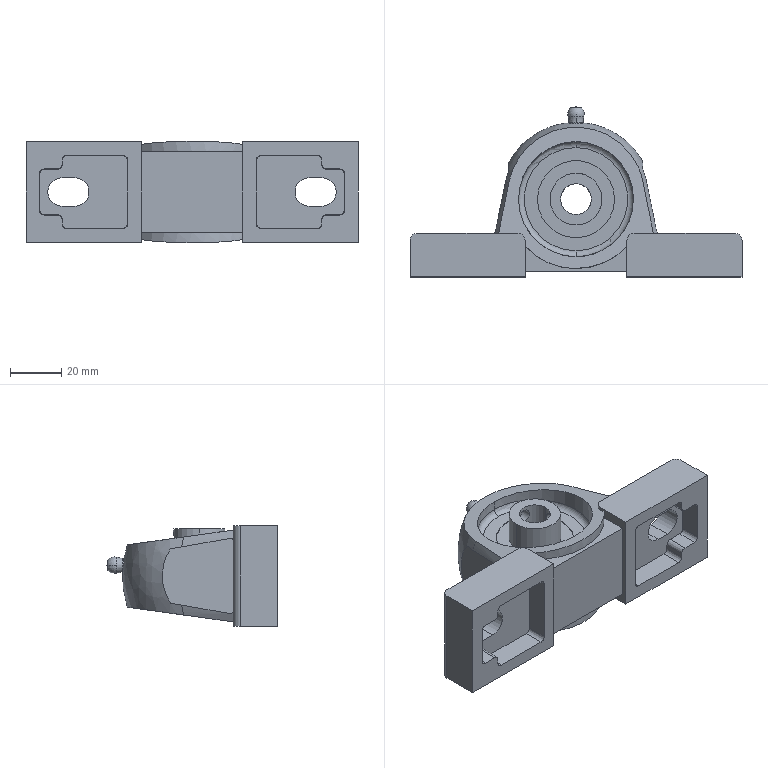Part | SolidWorks | features Revolution 5, Cut 3, Boss 2, CirPattern 2, ICE 2, RevCut 2, Extrusion 1, RefAxis 1, SweepCut 1 | 1 solid | 150 faces | box 129 x 66.06 x 39.46 mm | volume 93856 mm3 | plane 56 | cylinder 43 | sphere 22 | cone 16 | torus 8 | spline 5 | commonest cylinder face diameters 2 x6 6 x6 20.12 x6 29.96 x6 44.695 x6 5.134 x4